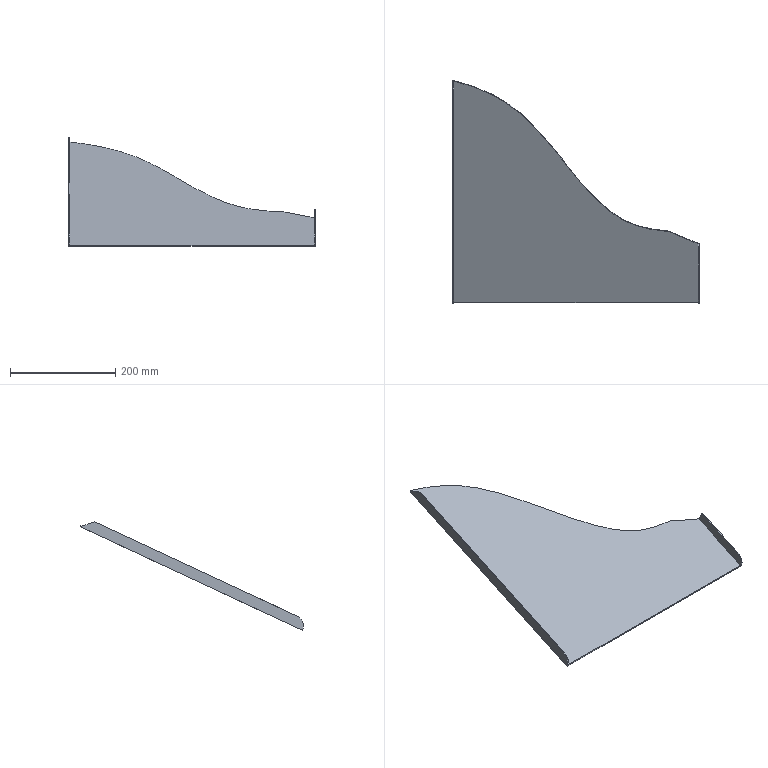Part | NX | features solid 2 | 1 solid | 15 faces | box 468.564 x 424.561 x 206.776 mm | volume 285219 mm3 | plane 12 | cylinder 2 | spline 1 | commonest cylinder face diameters 40 x2
STEP:
#1=CARTESIAN_POINT('',(216.564,-680.,-297.684));
#2=VERTEX_POINT('',#1);
#3=CARTESIAN_POINT('',(-248.,-680.,-297.684));
#4=VERTEX_POINT('',#3);
#5=CARTESIAN_POINT('',(188.564,-680.,-297.684));
#6=DIRECTION('',(1.,0.,0.));
#7=VECTOR('',#6,1000.);
#8=LINE('',#5,#7);
#9=EDGE_CURVE('',#2,#4,#8,.F.);
#10=ORIENTED_EDGE('',*,*,#9,.T.);
#11=CARTESIAN_POINT('',(-248.,-680.,-299.891));
#12=VERTEX_POINT('',#11);
#13=CARTESIAN_POINT('',(-248.,-680.,-430.));
#14=DIRECTION('',(0.,0.,1.));
#15=VECTOR('',#14,1000.);
#16=LINE('',#13,#15);
#17=EDGE_CURVE('',#4,#12,#16,.F.);
#18=ORIENTED_EDGE('',*,*,#17,.T.);
#19=CARTESIAN_POINT('',(216.564,-680.,-299.891));
#20=VERTEX_POINT('',#19);
#21=CARTESIAN_POINT('',(188.564,-680.,-299.891));
#22=DIRECTION('',(1.,0.,0.));
#23=VECTOR('',#22,1000.);
#24=LINE('',#21,#23);
#25=EDGE_CURVE('',#20,#12,#24,.F.);
#26=ORIENTED_EDGE('',*,*,#25,.F.);
#27=CARTESIAN_POINT('',(216.564,-680.,-430.));
#28=DIRECTION('',(0.,0.,1.));
#29=VECTOR('',#28,1000.);
#30=LINE('',#27,#29);
#31=EDGE_CURVE('',#2,#20,#30,.F.);
#32=ORIENTED_EDGE('',*,*,#31,.F.);
#33=EDGE_LOOP('',(#10,#18,#26,#32));
#34=FACE_BOUND('',#33,.T.);
#35=CARTESIAN_POINT('',(188.564,-680.,-430.));
#36=DIRECTION('',(0.,1.,0.));
#37=DIRECTION('',(-1.,0.,0.));
#38=AXIS2_PLACEMENT_3D('',#35,#36,#37);
#39=PLANE('',#38);
#40=ADVANCED_FACE('',(#34),#39,.F.);
#41=CARTESIAN_POINT('',(216.564,-567.897,-245.41));
#42=VERTEX_POINT('',#41);
#43=CARTESIAN_POINT('',(216.564,-570.845,-246.785));
#44=DIRECTION('',(0.,-0.9063,-0.4226));
#45=VECTOR('',#44,1000.);
#46=LINE('',#43,#45);
#47=EDGE_CURVE('',#42,#2,#46,.T.);
#48=ORIENTED_EDGE('',*,*,#47,.F.);
#49=CARTESIAN_POINT('',(192.998,-558.263,-240.917));
#50=VERTEX_POINT('',#49);
#51=CARTESIAN_POINT('',(248.564,-580.978,-251.51));
#52=CARTESIAN_POINT('',(218.564,-568.714,-245.791));
#53=CARTESIAN_POINT('',(188.564,-556.45,-240.072));
#54=CARTESIAN_POINT('',(186.796,-555.727,-239.735));
#55=CARTESIAN_POINT('',(185.026,-555.006,-239.399));
#56=CARTESIAN_POINT('',(183.703,-554.466,-239.147));
#57=CARTESIAN_POINT('',(181.508,-553.498,-238.696));
#58=CARTESIAN_POINT('',(179.151,-552.459,-238.211));
#59=CARTESIAN_POINT('',(174.521,-550.317,-237.212));
#60=CARTESIAN_POINT('',(169.002,-547.764,-236.022));
#61=CARTESIAN_POINT('',(167.553,-547.075,-235.701));
#62=CARTESIAN_POINT('',(165.721,-546.204,-235.294));
#63=CARTESIAN_POINT('',(165.233,-545.987,-235.193));
#64=CARTESIAN_POINT('',(164.588,-545.7,-235.06));
#65=CARTESIAN_POINT('',(164.056,-545.498,-234.965));
#66=CARTESIAN_POINT('',(162.357,-544.852,-234.664));
#67=CARTESIAN_POINT('',(160.35,-544.604,-234.548));
#68=CARTESIAN_POINT('',(159.573,-544.508,-234.504));
#69=CARTESIAN_POINT('',(158.413,-544.43,-234.467));
#70=CARTESIAN_POINT('',(157.06,-544.339,-234.425));
#71=CARTESIAN_POINT('',(156.465,-544.293,-234.403));
#72=CARTESIAN_POINT('',(154.804,-544.163,-234.343));
#73=CARTESIAN_POINT('',(152.593,-543.944,-234.24));
#74=CARTESIAN_POINT('',(148.836,-543.571,-234.067));
#75=CARTESIAN_POINT('',(144.885,-543.121,-233.857));
#76=CARTESIAN_POINT('',(136.794,-542.198,-233.426));
#77=CARTESIAN_POINT('',(129.623,-540.978,-232.857));
#78=CARTESIAN_POINT('',(113.905,-538.302,-231.61));
#79=CARTESIAN_POINT('',(100.072,-533.878,-229.547));
#80=CARTESIAN_POINT('',(85.036,-529.069,-227.304));
#81=CARTESIAN_POINT('',(72.615,-522.285,-224.141));
#82=CARTESIAN_POINT('',(60.937,-515.906,-221.166));
#83=CARTESIAN_POINT('',(48.09,-505.76,-216.435));
#84=CARTESIAN_POINT('',(37.227,-497.181,-212.435));
#85=CARTESIAN_POINT('',(26.181,-486.69,-207.543));
#86=CARTESIAN_POINT('',(16.265,-477.272,-203.151));
#87=CARTESIAN_POINT('',(5.983,-466.023,-197.905));
#88=CARTESIAN_POINT('',(-2.796,-456.418,-193.426));
#89=CARTESIAN_POINT('',(-12.946,-444.274,-187.763));
#90=CARTESIAN_POINT('',(-20.734,-434.955,-183.418));
#91=CARTESIAN_POINT('',(-31.105,-421.975,-177.366));
#92=CARTESIAN_POINT('',(-34.435,-417.807,-175.422));
#93=CARTESIAN_POINT('',(-40.051,-410.731,-172.122));
#94=CARTESIAN_POINT('',(-46.63,-402.44,-168.256));
#95=CARTESIAN_POINT('',(-48.988,-399.481,-166.876));
#96=CARTESIAN_POINT('',(-59.638,-386.11,-160.641));
#97=CARTESIAN_POINT('',(-67.079,-377.134,-156.456));
#98=CARTESIAN_POINT('',(-77.103,-365.041,-150.817));
#99=CARTESIAN_POINT('',(-85.894,-355.303,-146.276));
#100=CARTESIAN_POINT('',(-96.192,-343.895,-140.956));
#101=CARTESIAN_POINT('',(-105.983,-334.379,-136.519));
#102=CARTESIAN_POINT('',(-117.006,-323.667,-131.524));
#103=CARTESIAN_POINT('',(-127.887,-314.863,-127.418));
#104=CARTESIAN_POINT('',(-139.75,-305.265,-122.943));
#105=CARTESIAN_POINT('',(-151.704,-297.711,-119.42));
#106=CARTESIAN_POINT('',(-163.616,-290.185,-115.911));
#107=CARTESIAN_POINT('',(-177.719,-283.491,-112.789));
#108=CARTESIAN_POINT('',(-203.423,-271.29,-107.1));
#109=CARTESIAN_POINT('',(-234.262,-262.396,-102.952));
#110=CARTESIAN_POINT('',(-260.868,-254.722,-99.374));
#111=CARTESIAN_POINT('',(-293.238,-249.054,-96.731));
#112=CARTESIAN_POINT('',(-307.236,-246.603,-95.588));
#113=CARTESIAN_POINT('',(-323.289,-244.346,-94.536));
#114=CARTESIAN_POINT('',(-336.752,-242.454,-93.653));
#115=CARTESIAN_POINT('',(-353.561,-240.441,-92.715));
#116=CARTESIAN_POINT('',(-364.459,-239.135,-92.106));
#117=CARTESIAN_POINT('',(-383.92,-236.95,-91.087));
#118=CARTESIAN_POINT('',(-405.405,-234.537,-89.962));
#119=CARTESIAN_POINT('',(-414.287,-233.495,-89.476));
#120=CARTESIAN_POINT('',(-431.364,-231.492,-88.542));
#121=CARTESIAN_POINT('',(-444.588,-229.708,-87.71));
#122=CARTESIAN_POINT('',(-460.897,-227.508,-86.684));
#123=CARTESIAN_POINT('',(-474.746,-225.188,-85.602));
#124=CARTESIAN_POINT('',(-490.579,-222.535,-84.365));
#125=CARTESIAN_POINT('',(-504.673,-219.487,-82.944));
#126=CARTESIAN_POINT('',(-519.292,-216.325,-81.469));
#127=CARTESIAN_POINT('',(-534.302,-212.265,-79.576));
#128=CARTESIAN_POINT('',(-548.107,-208.53,-77.834));
#129=CARTESIAN_POINT('',(-563.609,-203.669,-75.568));
#130=CARTESIAN_POINT('',(-579.569,-198.665,-73.234));
#131=CARTESIAN_POINT('',(-592.283,-193.785,-70.959));
#132=CARTESIAN_POINT('',(-607.278,-188.029,-68.275));
#133=CARTESIAN_POINT('',(-619.815,-181.712,-65.329));
#134=CARTESIAN_POINT('',(-633.999,-174.564,-61.996));
#135=CARTESIAN_POINT('',(-645.657,-166.397,-58.187));
#136=B_SPLINE_CURVE_WITH_KNOTS('',2,(#51,#52,#53,#54,#55,#56,#57,#58,#59,#60,#61,#62,#63,#64,#65,#66,#67,#68,#69,#70,#71,#72,#73,#74,#75,#76,#77,#78,#79,#80,#81,#82,#83,#84,#85,#86,#87,#88,#89,#90,#91,#92,#93,#94,#95,#96,#97,#98,#99,#100,#101,#102,#103,#104,#105,#106,#107,#108,#109,#110,#111,#112,#113,#114,#115,#116,#117,#118,#119,#120,#121,#122,#123,#124,#125,#126,#127,#128,#129,#130,#131,#132,#133,#134,#135),.UNSPECIFIED.,.F.,.F.,(3,2,2,2,2,2,2,2,2,2,2,2,2,2,2,2,2,2,2,2,2,2,2,2,2,2,2,2,2,2,2,2,2,2,2,2,2,2,2,2,2,2,3),(-0.06626,0.,0.003906,0.007812,0.01562,0.02344,0.02604,0.02734,0.03125,0.0332,0.03516,0.03906,0.04688,0.0625,0.09375,0.125,0.1562,0.1875,0.2188,0.25,0.2812,0.2969,0.3125,0.3438,0.375,0.4062,0.4375,0.4688,0.5,0.5625,0.625,0.6562,0.6875,0.7188,0.75,0.7812,0.8125,0.8438,0.875,0.9062,0.9375,0.9688,1.),.PIECEWISE_BEZIER_KNOTS.);
#137=EDGE_CURVE('',#42,#50,#136,.T.);
#138=ORIENTED_EDGE('',*,*,#137,.T.);
#139=CARTESIAN_POINT('',(-250.,-258.158,-100.976));
#140=VERTEX_POINT('',#139);
#141=CARTESIAN_POINT('',(192.998,-558.263,-240.917));
#142=CARTESIAN_POINT('',(190.399,-557.2,-240.422));
#143=CARTESIAN_POINT('',(185.175,-555.126,-239.455));
#144=CARTESIAN_POINT('',(178.763,-552.284,-238.13));
#145=CARTESIAN_POINT('',(173.675,-549.923,-237.028));
#146=CARTESIAN_POINT('',(169.852,-548.168,-236.21));
#147=CARTESIAN_POINT('',(166.065,-546.336,-235.356));
#148=CARTESIAN_POINT('',(162.197,-544.676,-234.582));
#149=CARTESIAN_POINT('',(157.671,-544.397,-234.452));
#150=CARTESIAN_POINT('',(153.194,-544.018,-234.275));
#151=CARTESIAN_POINT('',(148.758,-543.552,-234.058));
#152=CARTESIAN_POINT('',(142.856,-542.905,-233.756));
#153=CARTESIAN_POINT('',(135.542,-541.961,-233.316));
#154=CARTESIAN_POINT('',(126.897,-540.551,-232.658));
#155=CARTESIAN_POINT('',(118.392,-538.847,-231.863));
#156=CARTESIAN_POINT('',(107.248,-536.163,-230.612));
#157=CARTESIAN_POINT('',(93.703,-531.997,-228.669));
#158=CARTESIAN_POINT('',(78.149,-525.528,-225.653));
#159=CARTESIAN_POINT('',(63.475,-517.194,-221.767));
#160=CARTESIAN_POINT('',(49.612,-507.205,-217.109));
#161=CARTESIAN_POINT('',(36.21,-496.055,-211.91));
#162=CARTESIAN_POINT('',(23.49,-484.296,-206.426));
#163=CARTESIAN_POINT('',(7.443,-467.991,-198.823));
#164=CARTESIAN_POINT('',(-11.275,-446.619,-188.857));
#165=CARTESIAN_POINT('',(-32.629,-420.174,-176.526));
#166=CARTESIAN_POINT('',(-53.659,-393.484,-164.08));
#167=CARTESIAN_POINT('',(-75.134,-367.144,-151.797));
#168=CARTESIAN_POINT('',(-97.866,-341.854,-140.004));
#169=CARTESIAN_POINT('',(-118.574,-322.211,-130.845));
#170=CARTESIAN_POINT('',(-136.664,-307.805,-124.127));
#171=CARTESIAN_POINT('',(-151.257,-297.71,-119.42));
#172=CARTESIAN_POINT('',(-166.604,-288.841,-115.284));
#173=CARTESIAN_POINT('',(-187.769,-278.525,-110.474));
#174=CARTESIAN_POINT('',(-215.315,-267.776,-105.461));
#175=CARTESIAN_POINT('',(-238.304,-261.096,-102.346));
#176=CARTESIAN_POINT('',(-250.,-258.158,-100.976));
#177=B_SPLINE_CURVE_WITH_KNOTS('',3,(#141,#142,#143,#144,#145,#146,#147,#148,#149,#150,#151,#152,#153,#154,#155,#156,#157,#158,#159,#160,#161,#162,#163,#164,#165,#166,#167,#168,#169,#170,#171,#172,#173,#174,#175,#176),.UNSPECIFIED.,.F.,.F.,(4,1,1,1,1,1,1,1,1,1,1,1,1,1,1,1,1,1,1,1,1,1,1,1,1,1,1,1,1,1,1,1,1,4),(0.,0.008555,0.01711,0.02139,0.02566,0.02994,0.03422,0.0385,0.04277,0.04705,0.05133,0.05988,0.06844,0.07699,0.08555,0.1027,0.1198,0.1369,0.154,0.1711,0.1882,0.2053,0.2395,0.2738,0.308,0.3422,0.3764,0.4106,0.4277,0.4449,0.462,0.4791,0.5133,0.5475),.UNSPECIFIED.);
#178=EDGE_CURVE('',#50,#140,#177,.T.);
#179=ORIENTED_EDGE('',*,*,#178,.T.);
#180=CARTESIAN_POINT('',(-250.,-259.971,-101.822));
#181=VERTEX_POINT('',#180);
#182=CARTESIAN_POINT('',(-250.,-570.845,-246.785));
#183=DIRECTION('',(0.,0.9063,0.4226));
#184=VECTOR('',#183,1000.);
#185=LINE('',#182,#184);
#186=EDGE_CURVE('',#140,#181,#185,.F.);
#187=ORIENTED_EDGE('',*,*,#186,.T.);
#188=CARTESIAN_POINT('',(-248.,-259.971,-101.822));
#189=VERTEX_POINT('',#188);
#190=CARTESIAN_POINT('',(-800.,-259.971,-101.822));
#191=DIRECTION('',(1.,0.,0.));
#192=VECTOR('',#191,1000.);
#193=LINE('',#190,#192);
#194=EDGE_CURVE('',#189,#181,#193,.F.);
#195=ORIENTED_EDGE('',*,*,#194,.F.);
#196=CARTESIAN_POINT('',(-248.,-570.845,-246.785));
#197=DIRECTION('',(0.,-0.9063,-0.4226));
#198=VECTOR('',#197,1000.);
#199=LINE('',#196,#198);
#200=EDGE_CURVE('',#189,#4,#199,.T.);
#201=ORIENTED_EDGE('',*,*,#200,.T.);
#202=ORIENTED_EDGE('',*,*,#9,.F.);
#203=EDGE_LOOP('',(#48,#138,#179,#187,#195,#201,#202));
#204=FACE_BOUND('',#203,.T.);
#205=CARTESIAN_POINT('',(-800.,-570.845,-246.785));
#206=DIRECTION('',(0.,-0.4226,0.9063));
#207=DIRECTION('',(0.,-0.9063,-0.4226));
#208=AXIS2_PLACEMENT_3D('',#205,#206,#207);
#209=PLANE('',#208);
#210=ADVANCED_FACE('',(#204),#209,.T.);
#211=ORIENTED_EDGE('',*,*,#137,.F.);
#212=CARTESIAN_POINT('',(216.564,-575.504,-229.096));
#213=VERTEX_POINT('',#212);
#214=CARTESIAN_POINT('',(216.564,-571.7,-237.253));
#215=DIRECTION('',(0.,0.4226,-0.9063));
#216=VECTOR('',#215,1000.);
#217=LINE('',#214,#216);
#218=EDGE_CURVE('',#42,#213,#217,.F.);
#219=ORIENTED_EDGE('',*,*,#218,.T.);
#220=CARTESIAN_POINT('',(218.564,-576.321,-229.477));
#221=VERTEX_POINT('',#220);
#222=CARTESIAN_POINT('',(216.564,-575.504,-229.096));
#223=CARTESIAN_POINT('',(217.231,-575.776,-229.223));
#224=CARTESIAN_POINT('',(217.898,-576.049,-229.35));
#225=CARTESIAN_POINT('',(218.564,-576.321,-229.477));
#226=B_SPLINE_CURVE_WITH_KNOTS('',3,(#222,#223,#224,#225),.UNSPECIFIED.,.F.,.F.,(4,4),(-0.01793,-0.01573),.UNSPECIFIED.);
#227=EDGE_CURVE('',#213,#221,#226,.T.);
#228=ORIENTED_EDGE('',*,*,#227,.T.);
#229=CARTESIAN_POINT('',(218.564,-567.869,-247.604));
#230=VERTEX_POINT('',#229);
#231=CARTESIAN_POINT('',(218.564,-572.095,-238.541));
#232=DIRECTION('',(0.,0.4226,-0.9063));
#233=VECTOR('',#232,1000.);
#234=LINE('',#231,#233);
#235=EDGE_CURVE('',#221,#230,#234,.T.);
#236=ORIENTED_EDGE('',*,*,#235,.T.);
#237=CARTESIAN_POINT('',(-248.,-257.82,-103.025));
#238=VERTEX_POINT('',#237);
#239=CARTESIAN_POINT('',(218.564,-567.869,-247.604));
#240=CARTESIAN_POINT('',(213.082,-565.628,-246.559));
#241=CARTESIAN_POINT('',(204.857,-562.271,-244.993));
#242=CARTESIAN_POINT('',(193.898,-557.777,-242.898));
#243=CARTESIAN_POINT('',(187.032,-555.005,-241.605));
#244=CARTESIAN_POINT('',(181.576,-552.707,-240.534));
#245=CARTESIAN_POINT('',(176.193,-550.251,-239.388));
#246=CARTESIAN_POINT('',(171.496,-548.075,-238.374));
#247=CARTESIAN_POINT('',(167.475,-546.199,-237.499));
#248=CARTESIAN_POINT('',(165.478,-545.232,-237.048));
#249=CARTESIAN_POINT('',(163.432,-544.369,-236.645));
#250=CARTESIAN_POINT('',(160.5,-543.661,-236.315));
#251=CARTESIAN_POINT('',(156.5,-543.499,-236.24));
#252=CARTESIAN_POINT('',(151.83,-543.024,-236.018));
#253=CARTESIAN_POINT('',(147.165,-542.539,-235.792));
#254=CARTESIAN_POINT('',(140.972,-541.832,-235.462));
#255=CARTESIAN_POINT('',(133.306,-540.787,-234.975));
#256=CARTESIAN_POINT('',(124.253,-539.217,-234.243));
#257=CARTESIAN_POINT('',(112.386,-536.683,-233.061));
#258=CARTESIAN_POINT('',(97.957,-532.644,-231.178));
#259=CARTESIAN_POINT('',(81.367,-526.228,-228.186));
#260=CARTESIAN_POINT('',(65.701,-517.823,-224.267));
#261=CARTESIAN_POINT('',(50.951,-507.43,-219.421));
#262=CARTESIAN_POINT('',(36.809,-495.753,-213.976));
#263=CARTESIAN_POINT('',(23.564,-483.537,-208.279));
#264=CARTESIAN_POINT('',(11.01,-470.767,-202.324));
#265=CARTESIAN_POINT('',(-4.942,-453.165,-194.116));
#266=CARTESIAN_POINT('',(-23.847,-430.382,-183.493));
#267=CARTESIAN_POINT('',(-45.847,-402.531,-170.505));
#268=CARTESIAN_POINT('',(-68.008,-374.802,-157.575));
#269=CARTESIAN_POINT('',(-91.274,-347.946,-145.052));
#270=CARTESIAN_POINT('',(-112.398,-326.919,-135.247));
#271=CARTESIAN_POINT('',(-130.883,-311.369,-127.996));
#272=CARTESIAN_POINT('',(-145.775,-300.447,-122.903));
#273=CARTESIAN_POINT('',(-161.368,-290.821,-118.414));
#274=CARTESIAN_POINT('',(-183.143,-279.663,-113.211));
#275=CARTESIAN_POINT('',(-211.719,-268.108,-107.823));
#276=CARTESIAN_POINT('',(-235.818,-260.933,-104.477));
#277=CARTESIAN_POINT('',(-248.,-257.82,-103.025));
#278=B_SPLINE_CURVE_WITH_KNOTS('',3,(#239,#240,#241,#242,#243,#244,#245,#246,#247,#248,#249,#250,#251,#252,#253,#254,#255,#256,#257,#258,#259,#260,#261,#262,#263,#264,#265,#266,#267,#268,#269,#270,#271,#272,#273,#274,#275,#276,#277),.UNSPECIFIED.,.F.,.F.,(4,1,1,1,1,1,1,1,1,1,1,1,1,1,1,1,1,1,1,1,1,1,1,1,1,1,1,1,1,1,1,1,1,1,1,1,4),(0.0329,0.05094,0.05995,0.06897,0.07348,0.07799,0.08701,0.08926,0.09152,0.09377,0.09602,0.1005,0.105,0.1096,0.1141,0.1231,0.1321,0.1411,0.1591,0.1772,0.1952,0.2133,0.2313,0.2493,0.2674,0.2854,0.3215,0.3575,0.3936,0.4297,0.4658,0.4838,0.5018,0.5199,0.5379,0.574,0.61),.UNSPECIFIED.);
#279=EDGE_CURVE('',#230,#238,#278,.T.);
#280=ORIENTED_EDGE('',*,*,#279,.T.);
#281=CARTESIAN_POINT('',(-248.,-258.056,-102.519));
#282=VERTEX_POINT('',#281);
#283=CARTESIAN_POINT('',(-248.,-258.665,-101.213));
#284=DIRECTION('',(0.,0.4226,-0.9063));
#285=VECTOR('',#284,1000.);
#286=LINE('',#283,#285);
#287=EDGE_CURVE('',#282,#238,#286,.T.);
#288=ORIENTED_EDGE('',*,*,#287,.F.);
#289=CARTESIAN_POINT('',(-250.,-257.313,-102.789));
#290=VERTEX_POINT('',#289);
#291=CARTESIAN_POINT('',(-248.,-258.056,-102.519));
#292=CARTESIAN_POINT('',(-248.666,-257.807,-102.609));
#293=CARTESIAN_POINT('',(-249.333,-257.559,-102.7));
#294=CARTESIAN_POINT('',(-250.,-257.313,-102.789));
#295=B_SPLINE_CURVE_WITH_KNOTS('',3,(#291,#292,#293,#294),.UNSPECIFIED.,.F.,.F.,(4,4),(0.,0.002151),.UNSPECIFIED.);
#296=EDGE_CURVE('',#282,#290,#295,.T.);
#297=ORIENTED_EDGE('',*,*,#296,.T.);
#298=CARTESIAN_POINT('',(-250.,-257.736,-101.883));
#299=DIRECTION('',(0.,0.4226,-0.9063));
#300=VECTOR('',#299,1000.);
#301=LINE('',#298,#300);
#302=EDGE_CURVE('',#140,#290,#301,.T.);
#303=ORIENTED_EDGE('',*,*,#302,.F.);
#304=ORIENTED_EDGE('',*,*,#178,.F.);
#305=EDGE_LOOP('',(#211,#219,#228,#236,#280,#288,#297,#303,#304));
#306=FACE_BOUND('',#305,.T.);
#307=CARTESIAN_POINT('',(218.564,-576.321,-229.477));
#308=CARTESIAN_POINT('',(218.564,-567.869,-247.604));
#309=CARTESIAN_POINT('',(215.671,-575.138,-228.926));
#310=CARTESIAN_POINT('',(215.671,-566.686,-247.052));
#311=CARTESIAN_POINT('',(209.883,-572.772,-227.823));
#312=CARTESIAN_POINT('',(209.883,-564.32,-245.949));
#313=CARTESIAN_POINT('',(201.204,-569.224,-226.168));
#314=CARTESIAN_POINT('',(201.204,-560.772,-244.294));
#315=CARTESIAN_POINT('',(193.964,-566.265,-224.788));
#316=CARTESIAN_POINT('',(193.964,-557.813,-242.914));
#317=CARTESIAN_POINT('',(189.27,-564.346,-223.893));
#318=CARTESIAN_POINT('',(189.27,-555.893,-242.019));
#319=CARTESIAN_POINT('',(187.092,-563.456,-223.478));
#320=CARTESIAN_POINT('',(187.092,-555.003,-241.604));
#321=CARTESIAN_POINT('',(186.024,-563.02,-223.275));
#322=CARTESIAN_POINT('',(186.024,-554.567,-241.401));
#323=CARTESIAN_POINT('',(185.064,-562.629,-223.093));
#324=CARTESIAN_POINT('',(185.064,-554.177,-241.219));
#325=CARTESIAN_POINT('',(184.529,-562.408,-222.99));
#326=CARTESIAN_POINT('',(184.529,-553.956,-241.116));
#327=CARTESIAN_POINT('',(183.885,-562.138,-222.864));
#328=CARTESIAN_POINT('',(183.885,-553.686,-240.99));
#329=CARTESIAN_POINT('',(183.17,-561.832,-222.721));
#330=CARTESIAN_POINT('',(183.17,-553.38,-240.847));
#331=CARTESIAN_POINT('',(182.38,-561.489,-222.561));
#332=CARTESIAN_POINT('',(182.38,-553.036,-240.687));
#333=CARTESIAN_POINT('',(181.827,-561.246,-222.448));
#334=CARTESIAN_POINT('',(181.827,-552.794,-240.574));
#335=CARTESIAN_POINT('',(181.422,-561.068,-222.365));
#336=CARTESIAN_POINT('',(181.422,-552.615,-240.491));
#337=CARTESIAN_POINT('',(181.214,-560.976,-222.322));
#338=CARTESIAN_POINT('',(181.214,-552.523,-240.448));
#339=CARTESIAN_POINT('',(180.731,-560.761,-222.222));
#340=CARTESIAN_POINT('',(180.731,-552.309,-240.348));
#341=CARTESIAN_POINT('',(179.737,-560.315,-222.014));
#342=CARTESIAN_POINT('',(179.737,-551.863,-240.14));
#343=CARTESIAN_POINT('',(178.028,-559.54,-221.652));
#344=CARTESIAN_POINT('',(178.028,-551.087,-239.778));
#345=CARTESIAN_POINT('',(176.136,-558.67,-221.247));
#346=CARTESIAN_POINT('',(176.136,-550.218,-239.373));
#347=CARTESIAN_POINT('',(174.807,-558.057,-220.961));
#348=CARTESIAN_POINT('',(174.807,-549.605,-239.087));
#349=CARTESIAN_POINT('',(173.722,-557.555,-220.727));
#350=CARTESIAN_POINT('',(173.722,-549.103,-238.853));
#351=CARTESIAN_POINT('',(171.907,-556.714,-220.335));
#352=CARTESIAN_POINT('',(171.907,-548.262,-238.461));
#353=CARTESIAN_POINT('',(170.251,-555.946,-219.976));
#354=CARTESIAN_POINT('',(170.251,-547.494,-238.102));
#355=CARTESIAN_POINT('',(168.966,-555.347,-219.697));
#356=CARTESIAN_POINT('',(168.966,-546.894,-237.823));
#357=CARTESIAN_POINT('',(168.324,-555.046,-219.557));
#358=CARTESIAN_POINT('',(168.324,-546.594,-237.683));
#359=CARTESIAN_POINT('',(167.958,-554.874,-219.476));
#360=CARTESIAN_POINT('',(167.958,-546.422,-237.603));
#361=CARTESIAN_POINT('',(167.774,-554.787,-219.436));
#362=CARTESIAN_POINT('',(167.774,-546.335,-237.562));
#363=CARTESIAN_POINT('',(167.644,-554.726,-219.407));
#364=CARTESIAN_POINT('',(167.644,-546.273,-237.533));
#365=CARTESIAN_POINT('',(167.539,-554.676,-219.384));
#366=CARTESIAN_POINT('',(167.539,-546.223,-237.51));
#367=CARTESIAN_POINT('',(166.902,-554.373,-219.243));
#368=CARTESIAN_POINT('',(166.902,-545.921,-237.369));
#369=CARTESIAN_POINT('',(166.383,-554.127,-219.128));
#370=CARTESIAN_POINT('',(166.383,-545.675,-237.254));
#371=CARTESIAN_POINT('',(165.815,-553.861,-219.004));
#372=CARTESIAN_POINT('',(165.815,-545.409,-237.13));
#373=CARTESIAN_POINT('',(165.497,-553.713,-218.935));
#374=CARTESIAN_POINT('',(165.497,-545.261,-237.061));
#375=CARTESIAN_POINT('',(165.299,-553.624,-218.893));
#376=CARTESIAN_POINT('',(165.299,-545.171,-237.02));
#377=CARTESIAN_POINT('',(165.258,-553.605,-218.885));
#378=CARTESIAN_POINT('',(165.258,-545.153,-237.011));
#379=CARTESIAN_POINT('',(165.027,-553.503,-218.837));
#380=CARTESIAN_POINT('',(165.027,-545.051,-236.963));
#381=CARTESIAN_POINT('',(164.806,-553.408,-218.793));
#382=CARTESIAN_POINT('',(164.806,-544.956,-236.919));
#383=CARTESIAN_POINT('',(164.252,-553.176,-218.685));
#384=CARTESIAN_POINT('',(164.252,-544.724,-236.811));
#385=CARTESIAN_POINT('',(163.511,-552.895,-218.554));
#386=CARTESIAN_POINT('',(163.511,-544.443,-236.68));
#387=CARTESIAN_POINT('',(162.389,-552.57,-218.402));
#388=CARTESIAN_POINT('',(162.389,-544.118,-236.528));
#389=CARTESIAN_POINT('',(161.44,-552.37,-218.309));
#390=CARTESIAN_POINT('',(161.44,-543.918,-236.435));
#391=CARTESIAN_POINT('',(160.609,-552.242,-218.249));
#392=CARTESIAN_POINT('',(160.609,-543.789,-236.375));
#393=CARTESIAN_POINT('',(159.9,-552.156,-218.209));
#394=CARTESIAN_POINT('',(159.9,-543.704,-236.335));
#395=CARTESIAN_POINT('',(158.989,-552.073,-218.17));
#396=CARTESIAN_POINT('',(158.989,-543.621,-236.296));
#397=CARTESIAN_POINT('',(157.627,-551.985,-218.129));
#398=CARTESIAN_POINT('',(157.627,-543.533,-236.255));
#399=CARTESIAN_POINT('',(156.851,-551.929,-218.103));
#400=CARTESIAN_POINT('',(156.851,-543.477,-236.229));
#401=CARTESIAN_POINT('',(156.345,-551.891,-218.086));
#402=CARTESIAN_POINT('',(156.345,-543.439,-236.212));
#403=CARTESIAN_POINT('',(155.371,-551.811,-218.048));
#404=CARTESIAN_POINT('',(155.371,-543.359,-236.174));
#405=CARTESIAN_POINT('',(154.23,-551.709,-218.001));
#406=CARTESIAN_POINT('',(154.23,-543.257,-236.127));
#407=CARTESIAN_POINT('',(153.126,-551.604,-217.952));
#408=CARTESIAN_POINT('',(153.126,-543.151,-236.078));
#409=CARTESIAN_POINT('',(152.286,-551.52,-217.913));
#410=CARTESIAN_POINT('',(152.286,-543.068,-236.039));
#411=CARTESIAN_POINT('',(151.532,-551.445,-217.877));
#412=CARTESIAN_POINT('',(151.532,-542.992,-236.004));
#413=CARTESIAN_POINT('',(150.163,-551.305,-217.812));
#414=CARTESIAN_POINT('',(150.163,-542.853,-235.938));
#415=CARTESIAN_POINT('',(148.204,-551.098,-217.716));
#416=CARTESIAN_POINT('',(148.204,-542.646,-235.842));
#417=CARTESIAN_POINT('',(145.821,-550.836,-217.593));
#418=CARTESIAN_POINT('',(145.821,-542.384,-235.72));
#419=CARTESIAN_POINT('',(142.529,-550.459,-217.418));
#420=CARTESIAN_POINT('',(142.529,-542.006,-235.544));
#421=CARTESIAN_POINT('',(138.501,-549.947,-217.179));
#422=CARTESIAN_POINT('',(138.501,-541.495,-235.305));
#423=CARTESIAN_POINT('',(134.634,-549.393,-216.92));
#424=CARTESIAN_POINT('',(134.634,-540.94,-235.047));
#425=CARTESIAN_POINT('',(131.605,-548.917,-216.699));
#426=CARTESIAN_POINT('',(131.605,-540.465,-234.825));
#427=CARTESIAN_POINT('',(129.431,-548.556,-216.53));
#428=CARTESIAN_POINT('',(129.431,-540.104,-234.656));
#429=CARTESIAN_POINT('',(126.968,-548.122,-216.328));
#430=CARTESIAN_POINT('',(126.968,-539.67,-234.454));
#431=CARTESIAN_POINT('',(123.822,-547.535,-216.054));
#432=CARTESIAN_POINT('',(123.822,-539.082,-234.18));
#433=CARTESIAN_POINT('',(119.908,-546.743,-215.685));
#434=CARTESIAN_POINT('',(119.908,-538.29,-233.811));
#435=CARTESIAN_POINT('',(115.316,-545.713,-215.205));
#436=CARTESIAN_POINT('',(115.316,-537.261,-233.331));
#437=CARTESIAN_POINT('',(110.806,-544.599,-214.685));
#438=CARTESIAN_POINT('',(110.806,-536.147,-232.811));
#439=CARTESIAN_POINT('',(106.397,-543.407,-214.129));
#440=CARTESIAN_POINT('',(106.397,-534.955,-232.255));
#441=CARTESIAN_POINT('',(102.762,-542.333,-213.629));
#442=CARTESIAN_POINT('',(102.762,-533.881,-231.755));
#443=CARTESIAN_POINT('',(99.975,-541.459,-213.221));
#444=CARTESIAN_POINT('',(99.975,-533.007,-231.347));
#445=CARTESIAN_POINT('',(96.848,-540.435,-212.743));
#446=CARTESIAN_POINT('',(96.848,-531.983,-230.87));
#447=CARTESIAN_POINT('',(91.661,-538.616,-211.895));
#448=CARTESIAN_POINT('',(91.661,-530.164,-230.022));
#449=CARTESIAN_POINT('',(84.469,-535.759,-210.563));
#450=CARTESIAN_POINT('',(84.469,-527.307,-228.689));
#451=CARTESIAN_POINT('',(78.382,-532.911,-209.235));
#452=CARTESIAN_POINT('',(78.382,-524.458,-227.361));
#453=CARTESIAN_POINT('',(74.495,-530.906,-208.3));
#454=CARTESIAN_POINT('',(74.495,-522.454,-226.426));
#455=CARTESIAN_POINT('',(72.543,-529.859,-207.812));
#456=CARTESIAN_POINT('',(72.543,-521.406,-225.938));
#457=CARTESIAN_POINT('',(70.789,-528.881,-207.356));
#458=CARTESIAN_POINT('',(70.789,-520.429,-225.482));
#459=CARTESIAN_POINT('',(67.144,-526.779,-206.375));
#460=CARTESIAN_POINT('',(67.144,-518.326,-224.501));
#461=CARTESIAN_POINT('',(61.621,-523.318,-204.762));
#462=CARTESIAN_POINT('',(61.621,-514.866,-222.888));
#463=CARTESIAN_POINT('',(55.908,-519.311,-202.893));
#464=CARTESIAN_POINT('',(55.908,-510.858,-221.019));
#465=CARTESIAN_POINT('',(52.041,-516.425,-201.547));
#466=CARTESIAN_POINT('',(52.041,-507.973,-219.674));
#467=CARTESIAN_POINT('',(50.408,-515.177,-200.966));
#468=CARTESIAN_POINT('',(50.408,-506.725,-219.092));
#469=CARTESIAN_POINT('',(49.118,-514.176,-200.499));
#470=CARTESIAN_POINT('',(49.118,-505.724,-218.625));
#471=CARTESIAN_POINT('',(48.082,-513.362,-200.119));
#472=CARTESIAN_POINT('',(48.082,-504.909,-218.245));
#473=CARTESIAN_POINT('',(47.294,-512.737,-199.828));
#474=CARTESIAN_POINT('',(47.294,-504.285,-217.954));
#475=CARTESIAN_POINT('',(46.167,-511.837,-199.408));
#476=CARTESIAN_POINT('',(46.167,-503.385,-217.534));
#477=CARTESIAN_POINT('',(44.783,-510.718,-198.886));
#478=CARTESIAN_POINT('',(44.783,-502.266,-217.012));
#479=CARTESIAN_POINT('',(42.552,-508.887,-198.032));
#480=CARTESIAN_POINT('',(42.552,-500.435,-216.159));
#481=CARTESIAN_POINT('',(39.762,-506.546,-196.941));
#482=CARTESIAN_POINT('',(39.762,-498.093,-215.067));
#483=CARTESIAN_POINT('',(36.402,-503.644,-195.587));
#484=CARTESIAN_POINT('',(36.402,-495.191,-213.713));
#485=CARTESIAN_POINT('',(33.039,-500.656,-194.194));
#486=CARTESIAN_POINT('',(33.039,-492.203,-212.32));
#487=CARTESIAN_POINT('',(30.216,-498.079,-192.993));
#488=CARTESIAN_POINT('',(30.216,-489.627,-211.119));
#489=CARTESIAN_POINT('',(27.981,-495.999,-192.022));
#490=CARTESIAN_POINT('',(27.981,-487.546,-210.149));
#491=CARTESIAN_POINT('',(26.23,-494.346,-191.252));
#492=CARTESIAN_POINT('',(26.23,-485.894,-209.378));
#493=CARTESIAN_POINT('',(24.753,-492.936,-190.594));
#494=CARTESIAN_POINT('',(24.753,-484.484,-208.72));
#495=CARTESIAN_POINT('',(22.702,-490.954,-189.67));
#496=CARTESIAN_POINT('',(22.702,-482.501,-207.796));
#497=CARTESIAN_POINT('',(20.153,-488.447,-188.501));
#498=CARTESIAN_POINT('',(20.153,-479.995,-206.627));
#499=CARTESIAN_POINT('',(17.066,-485.343,-187.054));
#500=CARTESIAN_POINT('',(17.066,-476.89,-205.18));
#501=CARTESIAN_POINT('',(13.964,-482.154,-185.567));
#502=CARTESIAN_POINT('',(13.964,-473.702,-203.693));
#503=CARTESIAN_POINT('',(10.848,-478.883,-184.041));
#504=CARTESIAN_POINT('',(10.848,-470.43,-202.167));
#505=CARTESIAN_POINT('',(8.487,-476.353,-182.861));
#506=CARTESIAN_POINT('',(8.487,-467.901,-200.988));
#507=CARTESIAN_POINT('',(6.925,-474.658,-182.071));
#508=CARTESIAN_POINT('',(6.925,-466.205,-200.197));
#509=CARTESIAN_POINT('',(5.842,-473.477,-181.52));
#510=CARTESIAN_POINT('',(5.842,-465.025,-199.647));
#511=CARTESIAN_POINT('',(4.775,-472.305,-180.974));
#512=CARTESIAN_POINT('',(4.775,-463.853,-199.1));
#513=CARTESIAN_POINT('',(3.386,-470.769,-180.257));
#514=CARTESIAN_POINT('',(3.386,-462.316,-198.384));
#515=CARTESIAN_POINT('',(0.624,-467.688,-178.821));
#516=CARTESIAN_POINT('',(0.624,-459.235,-196.947));
#517=CARTESIAN_POINT('',(-2.708,-463.903,-177.056));
#518=CARTESIAN_POINT('',(-2.708,-455.45,-195.182));
#519=CARTESIAN_POINT('',(-6.639,-459.344,-174.93));
#520=CARTESIAN_POINT('',(-6.639,-450.891,-193.056));
#521=CARTESIAN_POINT('',(-9.147,-456.399,-173.557));
#522=CARTESIAN_POINT('',(-9.147,-447.946,-191.683));
#523=CARTESIAN_POINT('',(-10.938,-454.275,-172.566));
#524=CARTESIAN_POINT('',(-10.938,-445.823,-190.693));
#525=CARTESIAN_POINT('',(-11.957,-453.062,-172.001));
#526=CARTESIAN_POINT('',(-11.957,-444.61,-190.127));
#527=CARTESIAN_POINT('',(-12.627,-452.262,-171.628));
#528=CARTESIAN_POINT('',(-12.627,-443.81,-189.754));
#529=CARTESIAN_POINT('',(-13.097,-451.7,-171.366));
#530=CARTESIAN_POINT('',(-13.097,-443.248,-189.492));
#531=CARTESIAN_POINT('',(-13.48,-451.241,-171.152));
#532=CARTESIAN_POINT('',(-13.48,-442.789,-189.278));
#533=CARTESIAN_POINT('',(-14.199,-450.379,-170.75));
#534=CARTESIAN_POINT('',(-14.199,-441.927,-188.876));
#535=CARTESIAN_POINT('',(-15.633,-448.652,-169.944));
#536=CARTESIAN_POINT('',(-15.633,-440.199,-188.07));
#537=CARTESIAN_POINT('',(-17.774,-446.058,-168.735));
#538=CARTESIAN_POINT('',(-17.774,-437.606,-186.861));
#539=CARTESIAN_POINT('',(-20.457,-442.782,-167.207));
#540=CARTESIAN_POINT('',(-20.457,-434.33,-185.333));
#541=CARTESIAN_POINT('',(-23.264,-439.331,-165.598));
#542=CARTESIAN_POINT('',(-23.264,-430.879,-183.724));
#543=CARTESIAN_POINT('',(-25.704,-436.313,-164.191));
#544=CARTESIAN_POINT('',(-25.704,-427.861,-182.317));
#545=CARTESIAN_POINT('',(-27.718,-433.81,-163.024));
#546=CARTESIAN_POINT('',(-27.718,-425.358,-181.15));
#547=CARTESIAN_POINT('',(-28.997,-432.216,-162.28));
#548=CARTESIAN_POINT('',(-28.997,-423.764,-180.406));
#549=CARTESIAN_POINT('',(-30.047,-430.905,-161.669));
#550=CARTESIAN_POINT('',(-30.047,-422.453,-179.795));
#551=CARTESIAN_POINT('',(-30.621,-430.188,-161.335));
#552=CARTESIAN_POINT('',(-30.621,-421.736,-179.461));
#553=CARTESIAN_POINT('',(-31.041,-429.662,-161.089));
#554=CARTESIAN_POINT('',(-31.041,-421.21,-179.215));
#555=CARTESIAN_POINT('',(-31.236,-429.418,-160.975));
#556=CARTESIAN_POINT('',(-31.236,-420.965,-179.101));
#557=CARTESIAN_POINT('',(-31.526,-429.056,-160.806));
#558=CARTESIAN_POINT('',(-31.526,-420.603,-178.933));
#559=CARTESIAN_POINT('',(-32.169,-428.25,-160.431));
#560=CARTESIAN_POINT('',(-32.169,-419.798,-178.557));
#561=CARTESIAN_POINT('',(-33.133,-427.041,-159.867));
#562=CARTESIAN_POINT('',(-33.133,-418.588,-177.993));
#563=CARTESIAN_POINT('',(-34.407,-425.441,-159.121));
#564=CARTESIAN_POINT('',(-34.407,-416.989,-177.247));
#565=CARTESIAN_POINT('',(-35.786,-423.707,-158.312));
#566=CARTESIAN_POINT('',(-35.786,-415.255,-176.438));
#567=CARTESIAN_POINT('',(-37.273,-421.837,-157.44));
#568=CARTESIAN_POINT('',(-37.273,-413.385,-175.566));
#569=CARTESIAN_POINT('',(-38.604,-420.16,-156.658));
#570=CARTESIAN_POINT('',(-38.604,-411.708,-174.785));
#571=CARTESIAN_POINT('',(-39.577,-418.935,-156.087));
#572=CARTESIAN_POINT('',(-39.577,-410.483,-174.213));
#573=CARTESIAN_POINT('',(-40.156,-418.205,-155.747));
#574=CARTESIAN_POINT('',(-40.156,-409.753,-173.873));
#575=CARTESIAN_POINT('',(-40.841,-417.342,-155.344));
#576=CARTESIAN_POINT('',(-40.841,-408.89,-173.471));
#577=CARTESIAN_POINT('',(-41.624,-416.356,-154.884));
#578=CARTESIAN_POINT('',(-41.624,-407.903,-173.01));
#579=CARTESIAN_POINT('',(-42.834,-414.831,-154.173));
#580=CARTESIAN_POINT('',(-42.834,-406.379,-172.3));
#581=CARTESIAN_POINT('',(-44.214,-413.093,-153.363));
#582=CARTESIAN_POINT('',(-44.214,-404.641,-171.489));
#583=CARTESIAN_POINT('',(-45.675,-411.253,-152.505));
#584=CARTESIAN_POINT('',(-45.675,-402.801,-170.631));
#585=CARTESIAN_POINT('',(-46.727,-409.93,-151.888));
#586=CARTESIAN_POINT('',(-46.727,-401.478,-170.014));
#587=CARTESIAN_POINT('',(-47.469,-408.997,-151.453));
#588=CARTESIAN_POINT('',(-47.469,-400.544,-169.579));
#589=CARTESIAN_POINT('',(-47.975,-408.36,-151.156));
#590=CARTESIAN_POINT('',(-47.975,-399.908,-169.282));
#591=CARTESIAN_POINT('',(-48.357,-407.879,-150.932));
#592=CARTESIAN_POINT('',(-48.357,-399.427,-169.058));
#593=CARTESIAN_POINT('',(-48.633,-407.533,-150.77));
#594=CARTESIAN_POINT('',(-48.633,-399.08,-168.896));
#595=CARTESIAN_POINT('',(-48.842,-407.27,-150.648));
#596=CARTESIAN_POINT('',(-48.842,-398.818,-168.774));
#597=CARTESIAN_POINT('',(-48.96,-407.122,-150.579));
#598=CARTESIAN_POINT('',(-48.96,-398.67,-168.705));
#599=CARTESIAN_POINT('',(-49.261,-406.745,-150.403));
#600=CARTESIAN_POINT('',(-49.261,-398.293,-168.529));
#601=CARTESIAN_POINT('',(-49.657,-406.248,-150.171));
#602=CARTESIAN_POINT('',(-49.657,-397.795,-168.297));
#603=CARTESIAN_POINT('',(-50.541,-405.139,-149.654));
#604=CARTESIAN_POINT('',(-50.541,-396.687,-167.78));
#605=CARTESIAN_POINT('',(-51.856,-403.493,-148.886));
#606=CARTESIAN_POINT('',(-51.856,-395.041,-167.013));
#607=CARTESIAN_POINT('',(-53.405,-401.558,-147.984));
#608=CARTESIAN_POINT('',(-53.405,-393.106,-166.11));
#609=CARTESIAN_POINT('',(-55.417,-399.051,-146.815));
#610=CARTESIAN_POINT('',(-55.417,-390.599,-164.941));
#611=CARTESIAN_POINT('',(-57.838,-396.045,-145.413));
#612=CARTESIAN_POINT('',(-57.838,-387.593,-163.54));
#613=CARTESIAN_POINT('',(-60.592,-392.646,-143.828));
#614=CARTESIAN_POINT('',(-60.592,-384.194,-161.954));
#615=CARTESIAN_POINT('',(-62.763,-389.984,-142.587));
#616=CARTESIAN_POINT('',(-62.763,-381.532,-160.713));
#617=CARTESIAN_POINT('',(-64.421,-387.961,-141.644));
#618=CARTESIAN_POINT('',(-64.421,-379.509,-159.77));
#619=CARTESIAN_POINT('',(-65.432,-386.733,-141.071));
#620=CARTESIAN_POINT('',(-65.432,-378.281,-159.197));
#621=CARTESIAN_POINT('',(-66.21,-385.791,-140.632));
#622=CARTESIAN_POINT('',(-66.21,-377.338,-158.758));
#623=CARTESIAN_POINT('',(-66.714,-385.182,-140.348));
#624=CARTESIAN_POINT('',(-66.714,-376.729,-158.474));
#625=CARTESIAN_POINT('',(-67.053,-384.771,-140.156));
#626=CARTESIAN_POINT('',(-67.053,-376.319,-158.282));
#627=CARTESIAN_POINT('',(-67.608,-384.103,-139.845));
#628=CARTESIAN_POINT('',(-67.608,-375.651,-157.971));
#629=CARTESIAN_POINT('',(-68.474,-383.061,-139.359));
#630=CARTESIAN_POINT('',(-68.474,-374.609,-157.485));
#631=CARTESIAN_POINT('',(-69.755,-381.527,-138.643));
#632=CARTESIAN_POINT('',(-69.755,-373.074,-156.769));
#633=CARTESIAN_POINT('',(-71.756,-379.143,-137.532));
#634=CARTESIAN_POINT('',(-71.756,-370.691,-155.658));
#635=CARTESIAN_POINT('',(-74.231,-376.222,-136.169));
#636=CARTESIAN_POINT('',(-74.231,-367.769,-154.296));
#637=CARTESIAN_POINT('',(-77.139,-372.831,-134.588));
#638=CARTESIAN_POINT('',(-77.139,-364.379,-152.715));
#639=CARTESIAN_POINT('',(-79.988,-369.552,-133.059));
#640=CARTESIAN_POINT('',(-79.988,-361.1,-151.186));
#641=CARTESIAN_POINT('',(-82.319,-366.906,-131.825));
#642=CARTESIAN_POINT('',(-82.319,-358.453,-149.952));
#643=CARTESIAN_POINT('',(-84.142,-364.858,-130.871));
#644=CARTESIAN_POINT('',(-84.142,-356.406,-148.997));
#645=CARTESIAN_POINT('',(-85.183,-363.698,-130.33));
#646=CARTESIAN_POINT('',(-85.183,-355.245,-148.456));
#647=CARTESIAN_POINT('',(-85.83,-362.98,-129.995));
#648=CARTESIAN_POINT('',(-85.83,-354.528,-148.121));
#649=CARTESIAN_POINT('',(-86.363,-362.391,-129.72));
#650=CARTESIAN_POINT('',(-86.363,-353.938,-147.846));
#651=CARTESIAN_POINT('',(-87.279,-361.38,-129.249));
#652=CARTESIAN_POINT('',(-87.279,-352.928,-147.375));
#653=CARTESIAN_POINT('',(-89.116,-359.367,-128.31));
#654=CARTESIAN_POINT('',(-89.116,-350.915,-146.436));
#655=CARTESIAN_POINT('',(-91.72,-356.553,-126.998));
#656=CARTESIAN_POINT('',(-91.72,-348.101,-145.124));
#657=CARTESIAN_POINT('',(-95.859,-352.165,-124.952));
#658=CARTESIAN_POINT('',(-95.859,-343.712,-143.078));
#659=CARTESIAN_POINT('',(-99.943,-347.962,-122.992));
#660=CARTESIAN_POINT('',(-99.943,-339.51,-141.118));
#661=CARTESIAN_POINT('',(-103.492,-344.424,-121.342));
#662=CARTESIAN_POINT('',(-103.492,-335.971,-139.468));
#663=CARTESIAN_POINT('',(-105.233,-342.716,-120.546));
#664=CARTESIAN_POINT('',(-105.233,-334.264,-138.672));
#665=CARTESIAN_POINT('',(-106.262,-341.715,-120.079));
#666=CARTESIAN_POINT('',(-106.262,-333.263,-138.205));
#667=CARTESIAN_POINT('',(-107.412,-340.603,-119.56));
#668=CARTESIAN_POINT('',(-107.412,-332.15,-137.686));
#669=CARTESIAN_POINT('',(-108.808,-339.267,-118.937));
#670=CARTESIAN_POINT('',(-108.808,-330.814,-137.063));
#671=CARTESIAN_POINT('',(-111.062,-337.136,-117.944));
#672=CARTESIAN_POINT('',(-111.062,-328.684,-136.07));
#673=CARTESIAN_POINT('',(-113.868,-334.538,-116.732));
#674=CARTESIAN_POINT('',(-113.868,-326.085,-134.858));
#675=CARTESIAN_POINT('',(-117.231,-331.505,-115.318));
#676=CARTESIAN_POINT('',(-117.231,-323.053,-133.444));
#677=CARTESIAN_POINT('',(-120.587,-328.564,-113.946));
#678=CARTESIAN_POINT('',(-120.587,-320.111,-132.072));
#679=CARTESIAN_POINT('',(-123.377,-326.188,-112.838));
#680=CARTESIAN_POINT('',(-123.377,-317.735,-130.964));
#681=CARTESIAN_POINT('',(-125.609,-324.33,-111.972));
#682=CARTESIAN_POINT('',(-125.609,-315.877,-130.098));
#683=CARTESIAN_POINT('',(-126.996,-323.192,-111.441));
#684=CARTESIAN_POINT('',(-126.996,-314.74,-129.567));
#685=CARTESIAN_POINT('',(-128.119,-322.282,-111.017));
#686=CARTESIAN_POINT('',(-128.119,-313.83,-129.143));
#687=CARTESIAN_POINT('',(-129.354,-321.289,-110.554));
#688=CARTESIAN_POINT('',(-129.354,-312.836,-128.68));
#689=CARTESIAN_POINT('',(-131.465,-319.614,-109.773));
#690=CARTESIAN_POINT('',(-131.465,-311.162,-127.899));
#691=CARTESIAN_POINT('',(-135.727,-316.319,-108.236));
#692=CARTESIAN_POINT('',(-135.727,-307.866,-126.362));
#693=CARTESIAN_POINT('',(-141.806,-311.868,-106.161));
#694=CARTESIAN_POINT('',(-141.806,-303.416,-124.287));
#695=CARTESIAN_POINT('',(-149.131,-306.902,-103.845));
#696=CARTESIAN_POINT('',(-149.131,-298.45,-121.972));
#697=CARTESIAN_POINT('',(-156.456,-302.334,-101.715));
#698=CARTESIAN_POINT('',(-156.456,-293.881,-119.841));
#699=CARTESIAN_POINT('',(-164.252,-297.888,-99.642));
#700=CARTESIAN_POINT('',(-164.252,-289.436,-117.768));
#701=CARTESIAN_POINT('',(-170.392,-294.681,-98.146));
#702=CARTESIAN_POINT('',(-170.392,-286.228,-116.272));
#703=CARTESIAN_POINT('',(-174.623,-292.587,-97.17));
#704=CARTESIAN_POINT('',(-174.623,-284.134,-115.296));
#705=CARTESIAN_POINT('',(-176.397,-291.727,-96.769));
#706=CARTESIAN_POINT('',(-176.397,-283.275,-114.895));
#707=CARTESIAN_POINT('',(-177.855,-291.033,-96.445));
#708=CARTESIAN_POINT('',(-177.855,-282.58,-114.571));
#709=CARTESIAN_POINT('',(-179.136,-290.428,-96.163));
#710=CARTESIAN_POINT('',(-179.136,-281.976,-114.289));
#711=CARTESIAN_POINT('',(-181.477,-289.338,-95.655));
#712=CARTESIAN_POINT('',(-181.477,-280.885,-113.781));
#713=CARTESIAN_POINT('',(-184.815,-287.825,-94.95));
#714=CARTESIAN_POINT('',(-184.815,-279.373,-113.076));
#715=CARTESIAN_POINT('',(-190.26,-285.446,-93.84));
#716=CARTESIAN_POINT('',(-190.26,-276.994,-111.966));
#717=CARTESIAN_POINT('',(-197.21,-282.573,-92.5));
#718=CARTESIAN_POINT('',(-197.21,-274.121,-110.627));
#719=CARTESIAN_POINT('',(-205.794,-279.279,-90.964));
#720=CARTESIAN_POINT('',(-205.794,-270.827,-109.091));
#721=CARTESIAN_POINT('',(-213.148,-276.664,-89.745));
#722=CARTESIAN_POINT('',(-213.148,-268.212,-107.871));
#723=CARTESIAN_POINT('',(-219.152,-274.651,-88.806));
#724=CARTESIAN_POINT('',(-219.152,-266.198,-106.932));
#725=CARTESIAN_POINT('',(-223.718,-273.178,-88.12));
#726=CARTESIAN_POINT('',(-223.718,-264.726,-106.246));
#727=CARTESIAN_POINT('',(-227.565,-271.986,-87.564));
#728=CARTESIAN_POINT('',(-227.565,-263.534,-105.69));
#729=CARTESIAN_POINT('',(-230.69,-271.047,-87.126));
#730=CARTESIAN_POINT('',(-230.69,-262.594,-105.252));
#731=CARTESIAN_POINT('',(-232.616,-270.479,-86.861));
#732=CARTESIAN_POINT('',(-232.616,-262.027,-104.987));
#733=CARTESIAN_POINT('',(-234.257,-270.004,-86.639));
#734=CARTESIAN_POINT('',(-234.257,-261.551,-104.765));
#735=CARTESIAN_POINT('',(-235.563,-269.629,-86.464));
#736=CARTESIAN_POINT('',(-235.563,-261.176,-104.591));
#737=CARTESIAN_POINT('',(-237.999,-268.939,-86.143));
#738=CARTESIAN_POINT('',(-237.999,-260.486,-104.269));
#739=CARTESIAN_POINT('',(-242.832,-267.607,-85.522));
#740=CARTESIAN_POINT('',(-242.832,-259.155,-103.648));
#741=CARTESIAN_POINT('',(-247.11,-266.491,-85.001));
#742=CARTESIAN_POINT('',(-247.11,-258.039,-103.128));
#743=CARTESIAN_POINT('',(-250.,-265.766,-84.663));
#744=CARTESIAN_POINT('',(-250.,-257.313,-102.789));
#745=B_SPLINE_SURFACE_WITH_KNOTS('',3,1,((#307,#308),(#309,#310),(#311,#312),(#313,#314),(#315,#316),(#317,#318),(#319,#320),(#321,#322),(#323,#324),(#325,#326),(#327,#328),(#329,#330),(#331,#332),(#333,#334),(#335,#336),(#337,#338),(#339,#340),(#341,#342),(#343,#344),(#345,#346),(#347,#348),(#349,#350),(#351,#352),(#353,#354),(#355,#356),(#357,#358),(#359,#360),(#361,#362),(#363,#364),(#365,#366),(#367,#368),(#369,#370),(#371,#372),(#373,#374),(#375,#376),(#377,#378),(#379,#380),(#381,#382),(#383,#384),(#385,#386),(#387,#388),(#389,#390),(#391,#392),(#393,#394),(#395,#396),(#397,#398),(#399,#400),(#401,#402),(#403,#404),(#405,#406),(#407,#408),(#409,#410),(#411,#412),(#413,#414),(#415,#416),(#417,#418),(#419,#420),(#421,#422),(#423,#424),(#425,#426),(#427,#428),(#429,#430),(#431,#432),(#433,#434),(#435,#436),(#437,#438),(#439,#440),(#441,#442),(#443,#444),(#445,#446),(#447,#448),(#449,#450),(#451,#452),(#453,#454),(#455,#456),(#457,#458),(#459,#460),(#461,#462),(#463,#464),(#465,#466),(#467,#468),(#469,#470),(#471,#472),(#473,#474),(#475,#476),(#477,#478),(#479,#480),(#481,#482),(#483,#484),(#485,#486),(#487,#488),(#489,#490),(#491,#492),(#493,#494),(#495,#496),(#497,#498),(#499,#500),(#501,#502),(#503,#504),(#505,#506),(#507,#508),(#509,#510),(#511,#512),(#513,#514),(#515,#516),(#517,#518),(#519,#520),(#521,#522),(#523,#524),(#525,#526),(#527,#528),(#529,#530),(#531,#532),(#533,#534),(#535,#536),(#537,#538),(#539,#540),(#541,#542),(#543,#544),(#545,#546),(#547,#548),(#549,#550),(#551,#552),(#553,#554),(#555,#556),(#557,#558),(#559,#560),(#561,#562),(#563,#564),(#565,#566),(#567,#568),(#569,#570),(#571,#572),(#573,#574),(#575,#576),(#577,#578),(#579,#580),(#581,#582),(#583,#584),(#585,#586),(#587,#588),(#589,#590),(#591,#592),(#593,#594),(#595,#596),(#597,#598),(#599,#600),(#601,#602),(#603,#604),(#605,#606),(#607,#608),(#609,#610),(#611,#612),(#613,#614),(#615,#616),(#617,#618),(#619,#620),(#621,#622),(#623,#624),(#625,#626),(#627,#628),(#629,#630),(#631,#632),(#633,#634),(#635,#636),(#637,#638),(#639,#640),(#641,#642),(#643,#644),(#645,#646),(#647,#648),(#649,#650),(#651,#652),(#653,#654),(#655,#656),(#657,#658),(#659,#660),(#661,#662),(#663,#664),(#665,#666),(#667,#668),(#669,#670),(#671,#672),(#673,#674),(#675,#676),(#677,#678),(#679,#680),(#681,#682),(#683,#684),(#685,#686),(#687,#688),(#689,#690),(#691,#692),(#693,#694),(#695,#696),(#697,#698),(#699,#700),(#701,#702),(#703,#704),(#705,#706),(#707,#708),(#709,#710),(#711,#712),(#713,#714),(#715,#716),(#717,#718),(#719,#720),(#721,#722),(#723,#724),(#725,#726),(#727,#728),(#729,#730),(#731,#732),(#733,#734),(#735,#736),(#737,#738),(#739,#740),(#741,#742),(#743,#744)),.SURF_OF_LINEAR_EXTRUSION.,.F.,.F.,.F.,(4,1,1,1,1,1,1,1,1,1,1,1,1,1,1,1,1,1,1,1,1,1,1,1,1,1,1,1,1,1,1,1,1,1,1,1,1,1,1,1,1,1,1,1,1,1,1,1,1,1,1,1,1,1,1,1,1,1,1,1,1,1,1,1,1,1,1,1,1,1,1,1,1,1,1,1,1,1,1,1,1,1,1,1,1,1,1,1,1,1,1,1,1,1,1,1,1,1,1,1,1,1,1,1,1,1,1,1,1,1,1,1,1,1,1,1,1,1,1,1,1,1,1,1,1,1,1,1,1,1,1,1,1,1,1,1,1,1,1,1,1,1,1,1,1,1,1,1,1,1,1,1,1,1,1,1,1,1,1,1,1,1,1,1,1,1,1,1,1,1,1,1,1,1,1,1,1,1,1,1,1,1,1,1,1,1,1,1,1,1,1,1,1,1,1,1,1,1,1,1,1,1,1,1,1,1,1,1,1,1,1,1,1,1,1,1,4),(2,2),(-0.03313,-0.02354,-0.01396,-0.00437,0.0004236,0.001622,0.00282,0.004019,0.004618,0.005217,0.006415,0.007015,0.007614,0.007913,0.008213,0.008812,0.01001,0.01241,0.0148,0.0154,0.016,0.0172,0.0196,0.0208,0.02199,0.02259,0.02289,0.02319,0.02349,0.02379,0.02439,0.02499,0.02559,0.02589,0.02604,0.02619,0.02649,0.02679,0.02799,0.02918,0.03038,0.03098,0.03158,0.03278,0.03398,0.03458,0.03518,0.03637,0.03757,0.03877,0.03937,0.03997,0.04117,0.04356,0.04596,0.04836,0.05315,0.05794,0.06034,0.06274,0.06513,0.06753,0.07232,0.07712,0.08191,0.08671,0.0915,0.0939,0.09629,0.1011,0.1107,0.1203,0.1227,0.1251,0.1274,0.1298,0.1394,0.149,0.1514,0.1538,0.155,0.1562,0.1574,0.1586,0.161,0.1634,0.1682,0.173,0.1778,0.1826,0.185,0.1874,0.1898,0.1922,0.197,0.2017,0.2065,0.2113,0.2161,0.2173,0.2185,0.2209,0.2233,0.2257,0.2353,0.2401,0.2449,0.2473,0.2485,0.2497,0.2503,0.2509,0.2521,0.2545,0.2593,0.2641,0.2689,0.2736,0.276,0.2784,0.2796,0.2808,0.2811,0.2814,0.282,0.2832,0.2856,0.288,0.2904,0.2928,0.2952,0.2964,0.297,0.2976,0.2988,0.3,0.3024,0.3048,0.3072,0.3084,0.3096,0.3108,0.3114,0.312,0.3126,0.3129,0.3132,0.3144,0.3168,0.3192,0.3216,0.3264,0.3312,0.336,0.3384,0.3408,0.342,0.3432,0.3438,0.3444,0.3456,0.3479,0.3503,0.3551,0.3599,0.3647,0.3695,0.3719,0.3743,0.3749,0.3755,0.3767,0.3791,0.3839,0.3887,0.3983,0.4031,0.4055,0.4067,0.4079,0.4103,0.4127,0.4175,0.4222,0.427,0.4318,0.4342,0.4366,0.4378,0.439,0.4414,0.4462,0.4558,0.4654,0.475,0.4846,0.4941,0.4965,0.4989,0.5001,0.5013,0.5037,0.5085,0.5133,0.5229,0.5325,0.5421,0.5469,0.5517,0.5565,0.5589,0.5613,0.5625,0.5637,0.566,0.5708,0.5804),(0.,1.),.UNSPECIFIED.);
#746=ADVANCED_FACE('',(#306),#745,.F.);
#747=CARTESIAN_POINT('',(-250.,-680.,-299.891));
#748=VERTEX_POINT('',#747);
#749=CARTESIAN_POINT('',(-250.,-570.,-248.597));
#750=DIRECTION('',(0.,0.9063,0.4226));
#751=VECTOR('',#750,1000.);
#752=LINE('',#749,#751);
#753=EDGE_CURVE('',#290,#748,#752,.F.);
#754=ORIENTED_EDGE('',*,*,#753,.F.);
#755=CARTESIAN_POINT('',(-248.,-257.313,-102.789));
#756=VERTEX_POINT('',#755);
#757=CARTESIAN_POINT('',(-250.,-257.313,-102.789));
#758=DIRECTION('',(1.,0.,0.));
#759=VECTOR('',#758,1000.);
#760=LINE('',#757,#759);
#761=EDGE_CURVE('',#290,#756,#760,.T.);
#762=ORIENTED_EDGE('',*,*,#761,.T.);
#763=CARTESIAN_POINT('',(-248.,-257.313,-102.789));
#764=DIRECTION('',(0.,-0.9063,-0.4226));
#765=VECTOR('',#764,1000.);
#766=LINE('',#763,#765);
#767=EDGE_CURVE('',#756,#238,#766,.T.);
#768=ORIENTED_EDGE('',*,*,#767,.T.);
#769=ORIENTED_EDGE('',*,*,#279,.F.);
#770=CARTESIAN_POINT('',(218.564,-680.,-299.891));
#771=VERTEX_POINT('',#770);
#772=CARTESIAN_POINT('',(218.564,-502.986,-217.348));
#773=DIRECTION('',(0.,-0.9063,-0.4226));
#774=VECTOR('',#773,1000.);
#775=LINE('',#772,#774);
#776=EDGE_CURVE('',#230,#771,#775,.T.);
#777=ORIENTED_EDGE('',*,*,#776,.T.);
#778=CARTESIAN_POINT('',(188.564,-680.,-299.891));
#779=DIRECTION('',(1.,0.,0.));
#780=VECTOR('',#779,1000.);
#781=LINE('',#778,#780);
#782=EDGE_CURVE('',#771,#20,#781,.F.);
#783=ORIENTED_EDGE('',*,*,#782,.T.);
#784=ORIENTED_EDGE('',*,*,#25,.T.);
#785=CARTESIAN_POINT('',(-250.,-680.,-299.891));
#786=DIRECTION('',(1.,0.,0.));
#787=VECTOR('',#786,1000.);
#788=LINE('',#785,#787);
#789=EDGE_CURVE('',#748,#12,#788,.T.);
#790=ORIENTED_EDGE('',*,*,#789,.F.);
#791=EDGE_LOOP('',(#754,#762,#768,#769,#777,#783,#784,#790));
#792=FACE_BOUND('',#791,.T.);
#793=CARTESIAN_POINT('',(-800.,-570.,-248.597));
#794=DIRECTION('',(0.,-0.4226,0.9063));
#795=DIRECTION('',(0.,-0.9063,-0.4226));
#796=AXIS2_PLACEMENT_3D('',#793,#794,#795);
#797=PLANE('',#796);
#798=ADVANCED_FACE('',(#792),#797,.F.);
#799=CARTESIAN_POINT('',(218.564,-670.326,-273.313));
#800=VERTEX_POINT('',#799);
#801=CARTESIAN_POINT('',(218.564,-661.874,-291.439));
#802=DIRECTION('',(1.,0.,0.));
#803=DIRECTION('',(0.,0.,-1.));
#804=AXIS2_PLACEMENT_3D('',#801,#802,#803);
#805=CIRCLE('',#804,20.);
#806=EDGE_CURVE('',#800,#771,#805,.T.);
#807=ORIENTED_EDGE('',*,*,#806,.T.);
#808=ORIENTED_EDGE('',*,*,#776,.F.);
#809=ORIENTED_EDGE('',*,*,#235,.F.);
#810=CARTESIAN_POINT('',(218.564,-564.057,-223.759));
#811=DIRECTION('',(0.,-0.9063,-0.4226));
#812=VECTOR('',#811,1000.);
#813=LINE('',#810,#812);
#814=EDGE_CURVE('',#221,#800,#813,.T.);
#815=ORIENTED_EDGE('',*,*,#814,.T.);
#816=EDGE_LOOP('',(#807,#808,#809,#815));
#817=FACE_BOUND('',#816,.T.);
#818=CARTESIAN_POINT('',(218.564,-503.831,-215.536));
#819=DIRECTION('',(1.,0.,0.));
#820=DIRECTION('',(0.,0.,-1.));
#821=AXIS2_PLACEMENT_3D('',#818,#819,#820);
#822=PLANE('',#821);
#823=ADVANCED_FACE('',(#817),#822,.T.);
#824=ORIENTED_EDGE('',*,*,#227,.F.);
#825=CARTESIAN_POINT('',(216.564,-670.326,-273.313));
#826=VERTEX_POINT('',#825);
#827=CARTESIAN_POINT('',(216.564,-564.057,-223.759));
#828=DIRECTION('',(0.,-0.9063,-0.4226));
#829=VECTOR('',#828,1000.);
#830=LINE('',#827,#829);
#831=EDGE_CURVE('',#213,#826,#830,.T.);
#832=ORIENTED_EDGE('',*,*,#831,.T.);
#833=CARTESIAN_POINT('',(188.564,-670.326,-273.313));
#834=DIRECTION('',(1.,0.,0.));
#835=VECTOR('',#834,1000.);
#836=LINE('',#833,#835);
#837=EDGE_CURVE('',#826,#800,#836,.T.);
#838=ORIENTED_EDGE('',*,*,#837,.T.);
#839=ORIENTED_EDGE('',*,*,#814,.F.);
#840=EDGE_LOOP('',(#824,#832,#838,#839));
#841=FACE_BOUND('',#840,.T.);
#842=CARTESIAN_POINT('',(188.564,-564.057,-223.759));
#843=DIRECTION('',(0.,0.4226,-0.9063));
#844=DIRECTION('',(0.,-0.9063,-0.4226));
#845=AXIS2_PLACEMENT_3D('',#842,#843,#844);
#846=PLANE('',#845);
#847=ADVANCED_FACE('',(#841),#846,.F.);
#848=ORIENTED_EDGE('',*,*,#218,.F.);
#849=ORIENTED_EDGE('',*,*,#47,.T.);
#850=ORIENTED_EDGE('',*,*,#31,.T.);
#851=CARTESIAN_POINT('',(216.564,-661.874,-291.439));
#852=DIRECTION('',(-1.,0.,0.));
#853=DIRECTION('',(0.,0.,1.));
#854=AXIS2_PLACEMENT_3D('',#851,#852,#853);
#855=CIRCLE('',#854,20.);
#856=EDGE_CURVE('',#20,#826,#855,.T.);
#857=ORIENTED_EDGE('',*,*,#856,.T.);
#858=ORIENTED_EDGE('',*,*,#831,.F.);
#859=EDGE_LOOP('',(#848,#849,#850,#857,#858));
#860=FACE_BOUND('',#859,.T.);
#861=CARTESIAN_POINT('',(216.564,-555.605,-241.885));
#862=DIRECTION('',(-1.,0.,0.));
#863=DIRECTION('',(0.,0.,1.));
#864=AXIS2_PLACEMENT_3D('',#861,#862,#863);
#865=PLANE('',#864);
#866=ADVANCED_FACE('',(#860),#865,.T.);
#867=ORIENTED_EDGE('',*,*,#806,.F.);
#868=ORIENTED_EDGE('',*,*,#837,.F.);
#869=ORIENTED_EDGE('',*,*,#856,.F.);
#870=ORIENTED_EDGE('',*,*,#782,.F.);
#871=EDGE_LOOP('',(#867,#868,#869,#870));
#872=FACE_BOUND('',#871,.T.);
#873=CARTESIAN_POINT('',(188.564,-661.874,-291.439));
#874=DIRECTION('',(1.,0.,0.));
#875=DIRECTION('',(0.,0.,-1.));
#876=AXIS2_PLACEMENT_3D('',#873,#874,#875);
#877=CYLINDRICAL_SURFACE('',#876,20.);
#878=ADVANCED_FACE('',(#872),#877,.T.);
#879=ORIENTED_EDGE('',*,*,#753,.T.);
#880=CARTESIAN_POINT('',(-250.,-670.326,-273.313));
#881=VERTEX_POINT('',#880);
#882=CARTESIAN_POINT('',(-250.,-661.874,-291.439));
#883=DIRECTION('',(-1.,0.,0.));
#884=DIRECTION('',(0.,0.,1.));
#885=AXIS2_PLACEMENT_3D('',#882,#883,#884);
#886=CIRCLE('',#885,20.);
#887=EDGE_CURVE('',#748,#881,#886,.T.);
#888=ORIENTED_EDGE('',*,*,#887,.T.);
#889=CARTESIAN_POINT('',(-250.,-283.892,-93.115));
#890=VERTEX_POINT('',#889);
#891=CARTESIAN_POINT('',(-250.,-265.766,-84.663));
#892=DIRECTION('',(0.,-0.9063,-0.4226));
#893=VECTOR('',#892,1000.);
#894=LINE('',#891,#893);
#895=EDGE_CURVE('',#890,#881,#894,.T.);
#896=ORIENTED_EDGE('',*,*,#895,.F.);
#897=CARTESIAN_POINT('',(-250.,-257.313,-102.789));
#898=DIRECTION('',(0.,-0.9397,0.342));
#899=VECTOR('',#898,1000.);
#900=LINE('',#897,#899);
#901=EDGE_CURVE('',#890,#181,#900,.F.);
#902=ORIENTED_EDGE('',*,*,#901,.T.);
#903=ORIENTED_EDGE('',*,*,#186,.F.);
#904=ORIENTED_EDGE('',*,*,#302,.T.);
#905=EDGE_LOOP('',(#879,#888,#896,#902,#903,#904));
#906=FACE_BOUND('',#905,.T.);
#907=CARTESIAN_POINT('',(-250.,-560.,-105.));
#908=DIRECTION('',(1.,0.,0.));
#909=DIRECTION('',(0.,0.,-1.));
#910=AXIS2_PLACEMENT_3D('',#907,#908,#909);
#911=PLANE('',#910);
#912=ADVANCED_FACE('',(#906),#911,.F.);
#913=CARTESIAN_POINT('',(-248.,-283.892,-93.115));
#914=VERTEX_POINT('',#913);
#915=CARTESIAN_POINT('',(-248.,-257.313,-102.789));
#916=DIRECTION('',(0.,0.9397,-0.342));
#917=VECTOR('',#916,1000.);
#918=LINE('',#915,#917);
#919=EDGE_CURVE('',#189,#914,#918,.F.);
#920=ORIENTED_EDGE('',*,*,#919,.F.);
#921=ORIENTED_EDGE('',*,*,#194,.T.);
#922=ORIENTED_EDGE('',*,*,#901,.F.);
#923=CARTESIAN_POINT('',(-250.,-283.892,-93.115));
#924=DIRECTION('',(1.,0.,0.));
#925=VECTOR('',#924,1000.);
#926=LINE('',#923,#925);
#927=EDGE_CURVE('',#914,#890,#926,.F.);
#928=ORIENTED_EDGE('',*,*,#927,.F.);
#929=EDGE_LOOP('',(#920,#921,#922,#928));
#930=FACE_BOUND('',#929,.T.);
#931=CARTESIAN_POINT('',(-250.,-257.313,-102.789));
#932=DIRECTION('',(0.,-0.342,-0.9397));
#933=DIRECTION('',(0.,0.9397,-0.342));
#934=AXIS2_PLACEMENT_3D('',#931,#932,#933);
#935=PLANE('',#934);
#936=ADVANCED_FACE('',(#930),#935,.F.);
#937=ORIENTED_EDGE('',*,*,#887,.F.);
#938=ORIENTED_EDGE('',*,*,#789,.T.);
#939=CARTESIAN_POINT('',(-248.,-670.326,-273.313));
#940=VERTEX_POINT('',#939);
#941=CARTESIAN_POINT('',(-248.,-661.874,-291.439));
#942=DIRECTION('',(-1.,0.,0.));
#943=DIRECTION('',(0.,0.,1.));
#944=AXIS2_PLACEMENT_3D('',#941,#942,#943);
#945=CIRCLE('',#944,20.);
#946=EDGE_CURVE('',#940,#12,#945,.F.);
#947=ORIENTED_EDGE('',*,*,#946,.F.);
#948=CARTESIAN_POINT('',(-250.,-670.326,-273.313));
#949=DIRECTION('',(1.,0.,0.));
#950=VECTOR('',#949,1000.);
#951=LINE('',#948,#950);
#952=EDGE_CURVE('',#881,#940,#951,.T.);
#953=ORIENTED_EDGE('',*,*,#952,.F.);
#954=EDGE_LOOP('',(#937,#938,#947,#953));
#955=FACE_BOUND('',#954,.T.);
#956=CARTESIAN_POINT('',(-250.,-661.874,-291.439));
#957=DIRECTION('',(-1.,0.,0.));
#958=DIRECTION('',(0.,0.,1.));
#959=AXIS2_PLACEMENT_3D('',#956,#957,#958);
#960=CYLINDRICAL_SURFACE('',#959,20.);
#961=ADVANCED_FACE('',(#955),#960,.T.);
#962=ORIENTED_EDGE('',*,*,#17,.F.);
#963=ORIENTED_EDGE('',*,*,#200,.F.);
#964=ORIENTED_EDGE('',*,*,#919,.T.);
#965=CARTESIAN_POINT('',(-248.,-265.766,-84.663));
#966=DIRECTION('',(0.,-0.9063,-0.4226));
#967=VECTOR('',#966,1000.);
#968=LINE('',#965,#967);
#969=EDGE_CURVE('',#914,#940,#968,.T.);
#970=ORIENTED_EDGE('',*,*,#969,.T.);
#971=ORIENTED_EDGE('',*,*,#946,.T.);
#972=EDGE_LOOP('',(#962,#963,#964,#970,#971));
#973=FACE_BOUND('',#972,.T.);
#974=CARTESIAN_POINT('',(-248.,-257.313,-102.789));
#975=DIRECTION('',(-1.,0.,0.));
#976=DIRECTION('',(0.,0.,1.));
#977=AXIS2_PLACEMENT_3D('',#974,#975,#976);
#978=PLANE('',#977);
#979=ADVANCED_FACE('',(#973),#978,.F.);
#980=ORIENTED_EDGE('',*,*,#969,.F.);
#981=ORIENTED_EDGE('',*,*,#927,.T.);
#982=ORIENTED_EDGE('',*,*,#895,.T.);
#983=ORIENTED_EDGE('',*,*,#952,.T.);
#984=EDGE_LOOP('',(#980,#981,#982,#983));
#985=FACE_BOUND('',#984,.T.);
#986=CARTESIAN_POINT('',(-250.,-265.766,-84.663));
#987=DIRECTION('',(0.,0.4226,-0.9063));
#988=DIRECTION('',(0.,-0.9063,-0.4226));
#989=AXIS2_PLACEMENT_3D('',#986,#987,#988);
#990=PLANE('',#989);
#991=ADVANCED_FACE('',(#985),#990,.F.);
#992=CARTESIAN_POINT('',(-248.,-257.313,-102.789));
#993=DIRECTION('',(0.,0.9397,-0.342));
#994=VECTOR('',#993,1000.);
#995=LINE('',#992,#994);
#996=EDGE_CURVE('',#756,#282,#995,.F.);
#997=ORIENTED_EDGE('',*,*,#996,.T.);
#998=ORIENTED_EDGE('',*,*,#287,.T.);
#999=ORIENTED_EDGE('',*,*,#767,.F.);
#1000=EDGE_LOOP('',(#997,#998,#999));
#1001=FACE_BOUND('',#1000,.T.);
#1002=CARTESIAN_POINT('',(-248.,-257.313,-102.789));
#1003=DIRECTION('',(-1.,0.,0.));
#1004=DIRECTION('',(0.,0.,1.));
#1005=AXIS2_PLACEMENT_3D('',#1002,#1003,#1004);
#1006=PLANE('',#1005);
#1007=ADVANCED_FACE('',(#1001),#1006,.F.);
#1008=ORIENTED_EDGE('',*,*,#296,.F.);
#1009=ORIENTED_EDGE('',*,*,#996,.F.);
#1010=ORIENTED_EDGE('',*,*,#761,.F.);
#1011=EDGE_LOOP('',(#1008,#1009,#1010));
#1012=FACE_BOUND('',#1011,.T.);
#1013=CARTESIAN_POINT('',(-250.,-257.313,-102.789));
#1014=DIRECTION('',(0.,-0.342,-0.9397));
#1015=DIRECTION('',(0.,0.9397,-0.342));
#1016=AXIS2_PLACEMENT_3D('',#1013,#1014,#1015);
#1017=PLANE('',#1016);
#1018=ADVANCED_FACE('',(#1012),#1017,.F.);
#1019=CLOSED_SHELL('',(#40,#210,#746,#798,#823,#847,#866,#878,#912,#936,#961,#979,#991,#1007,#1018));
#1020=MANIFOLD_SOLID_BREP('',#1019);
#1021=(LENGTH_UNIT()NAMED_UNIT(*)SI_UNIT(.MILLI.,.METRE.));
#1022=UNCERTAINTY_MEASURE_WITH_UNIT(LENGTH_MEASURE(0.0508),#1021,'','');
#1023=(NAMED_UNIT(*)PLANE_ANGLE_UNIT()SI_UNIT($,.RADIAN.));
#1024=(NAMED_UNIT(*)SI_UNIT($,.STERADIAN.)SOLID_ANGLE_UNIT());
#1025=(GEOMETRIC_REPRESENTATION_CONTEXT(3)GLOBAL_UNCERTAINTY_ASSIGNED_CONTEXT((#1022))GLOBAL_UNIT_ASSIGNED_CONTEXT((#1021,#1023,#1024))REPRESENTATION_CONTEXT('',''));
#1026=ADVANCED_BREP_SHAPE_REPRESENTATION('',(#1020),#1025);